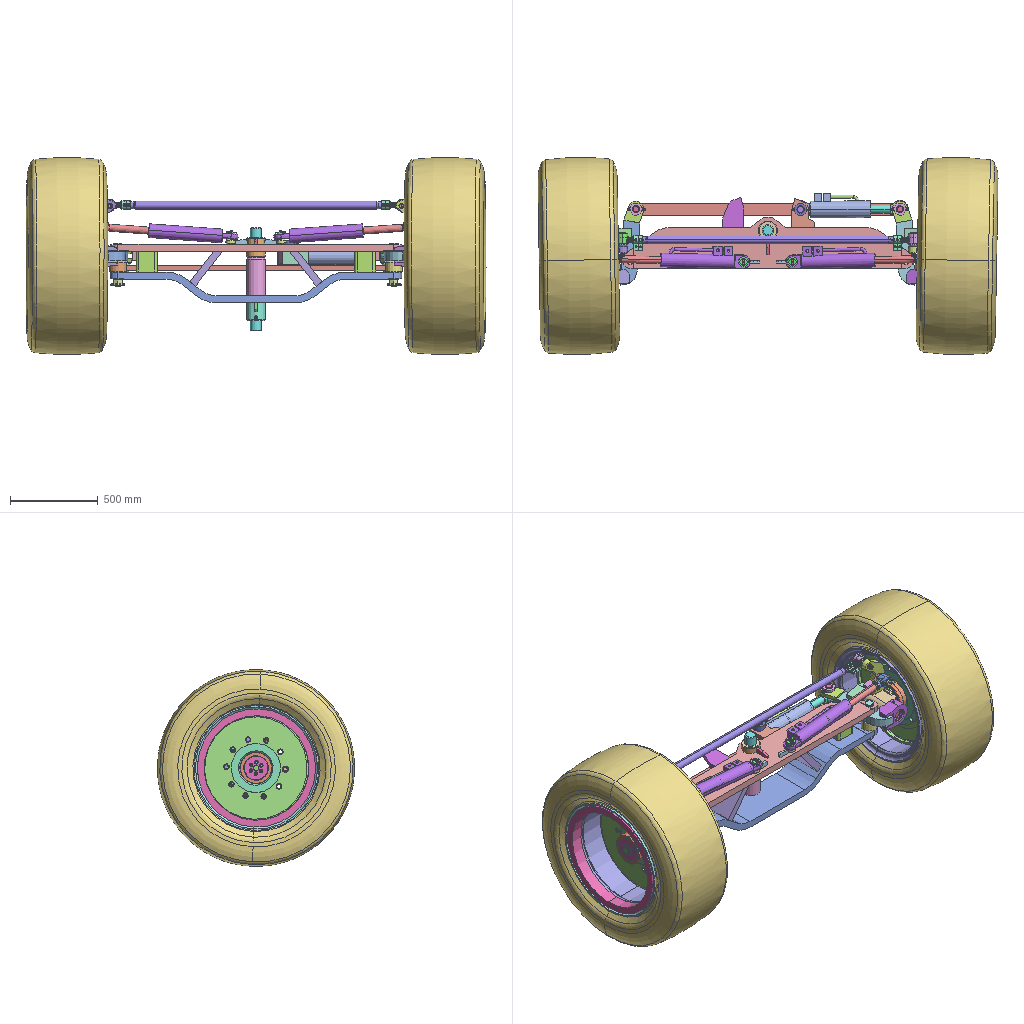Assembly | SolidWorks | 108 different items | 254 placed | box 2615 x 1120 x 1117 mm
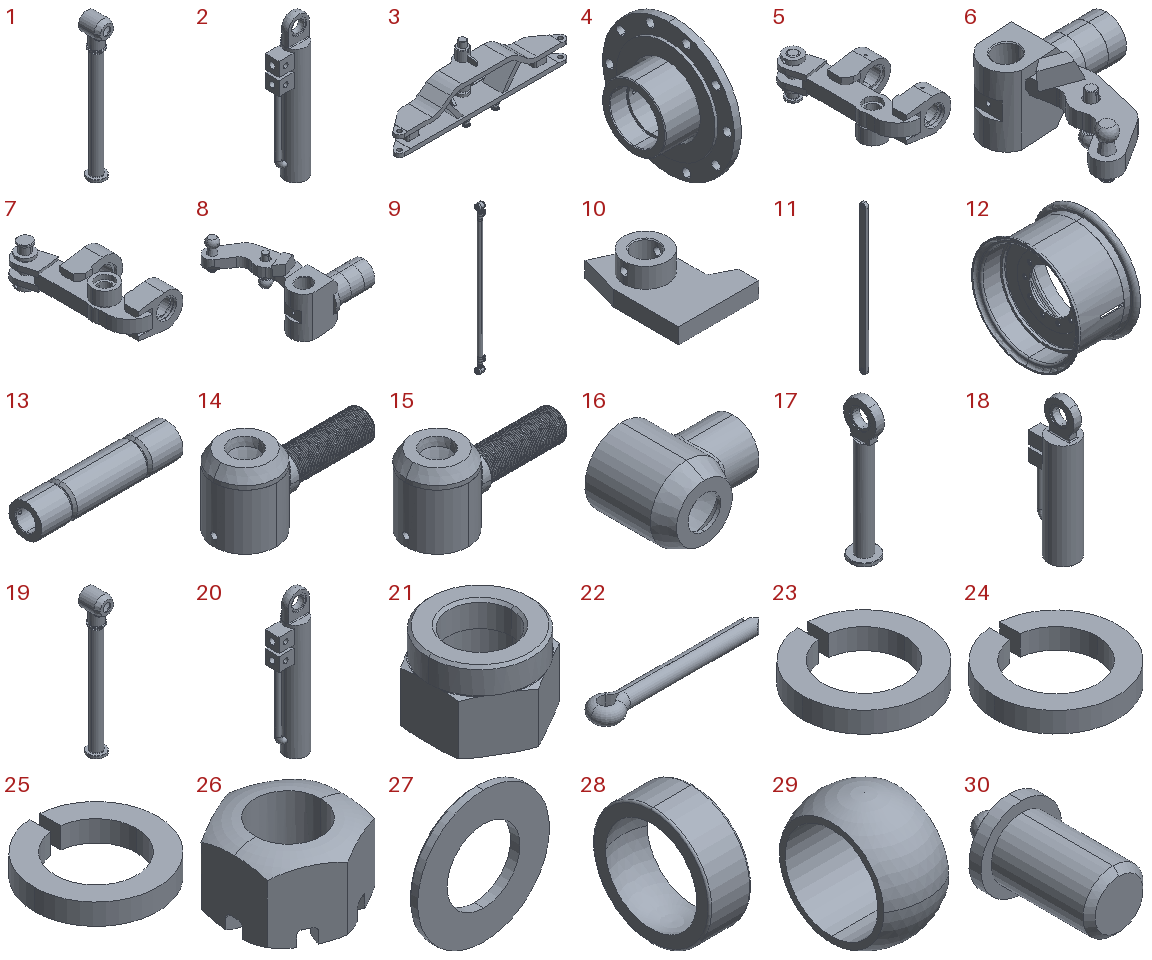Parts list (item | name | quantity | parent item | size | volume | features):
1 | (subassembly) | x1 | - | 65 x 84.5 x 521.5 mm | 755926 mm3 | features AEMSimFeature 1
2 | (subassembly) | x1 | - | 124 x 78 x 509 mm | 1093620 mm3 | features AEMSimFeature 1
3 | (subassembly) | x1 | - | 1658 x 403.509 x 586 mm | 38283555 mm3 | -
4 | (subassembly) | x2 | - | 164 x 375 x 375 mm | 3788319 mm3 | features AEMSimFeature 1
5 | (subassembly) | x1 | - | 241.001 x 479.989 x 157 mm | 4305652 mm3 | features Cut 2, RefAxis 2, RevCut 2, AEMSimFeature 1
6 | (subassembly) | x1 | - | 314 x 375 x 193.9 mm | 3181151 mm3 | features CompositeCurve 2, AEMSimFeature 1
7 | (subassembly) | x1 | - | 241.001 x 479.989 x 157 mm | 4310466 mm3 | features Cut 2, RefAxis 2, RevCut 2, AEMSimFeature 1
8 | (subassembly) | x1 | - | 314 x 375 x 193.9 mm | 3181178 mm3 | features CompositeCurve 2, AEMSimFeature 1
9 | (subassembly) | x1 | - | 103 x 64 x 1722 mm | 2094489 mm3 | features ReferencePattern 2, MirrorCompFeat 1
10 | (subassembly) | x1 | in 3 | 129 x 168.47 x 72 mm | 470442 mm3 | features AEMSimFeature 1
11 | (subassembly) | x1 | - | 30 x 77.5 x 1570 mm | 3189069 mm3 | features MirrorCompFeat 1, ReferencePattern 1
12 | (subassembly) | x2 | - | 410 x 711 x 711 mm | 14022631 mm3 | features AEMSimFeature 1
13 | (subassembly) | x1 | in 3 | 462 x 108 x 108 mm | 2151282 mm3 | features AEMSimFeature 1
14 | (subassembly) | x1 | in 9 | 152 x 64 x 82 mm | 214703 mm3 | -
15 | (subassembly) | x1 | in 9 | 152 x 64 x 82 mm | 214559 mm3 | -
16 | (subassembly) | x2 | in 1, 19 | 97.5 x 84.5 x 65 mm | 175742 mm3 | features AEMSimFeature 1
17 | (subassembly) | x1 | - | 80 x 100 x 410 mm | 667768 mm3 | features AEMSimFeature 1
18 | (subassembly) | x1 | - | 95 x 142.5 x 448 mm | 1129896 mm3 | features AEMSimFeature 1
19 | (subassembly) | x1 | - | 65 x 84.5 x 521.5 mm | 755926 mm3 | features AEMSimFeature 1
20 | (subassembly) | x1 | - | 124 x 78 x 509 mm | 1093620 mm3 | features AEMSimFeature 1
21 | - | x3 | - | 15.68 x 17.77 x 11.9 mm | 1480 mm3 | features Cut 3, Boss 1, Chamfer 1, Extrusion 1
22 | - | x2 | - | 83 x 15 x 8 mm | 4081 mm3 | features Cut 1, Sweep 1
23 | - | x12 | - | 18.367 x 18.334 x 3.1 mm | 444.091 mm3 | features Extrusion 1
24 | - | x2 | - | 30.149 x 30.097 x 5 mm | 1905 mm3 | features Extrusion 1
25 | - | x4 | - | 12.277 x 12.254 x 2.1 mm | 135.755 mm3 | features Extrusion 1
26 | - | x2 | - | 46 x 50.85 x 34.366 mm | 35234 mm3 | features CirPattern 1, Extrusion 1, Fillet 1, HoleWzd 1, ICE 1, RefAxis 1, RevCut 1
27 | - | x2 | - | 56 x 4 x 56 mm | 6746 mm3 | features Revolution 1
28 | - | x2 | in 17, 18 | 22 x 62 x 62 mm | 20588 mm3 | features Fillet 1, Revolution 1
29 | - | x2 | in 3, 5 | 28 x 53 x 53 mm | 20840 mm3 | features Revolution 1
30 | - | x8 | in 11 | 13.4 x 23.7 x 13.4 mm | 1610 mm3 | features Chamfer 1, Extrusion 1, ICE 1, Revolution 1
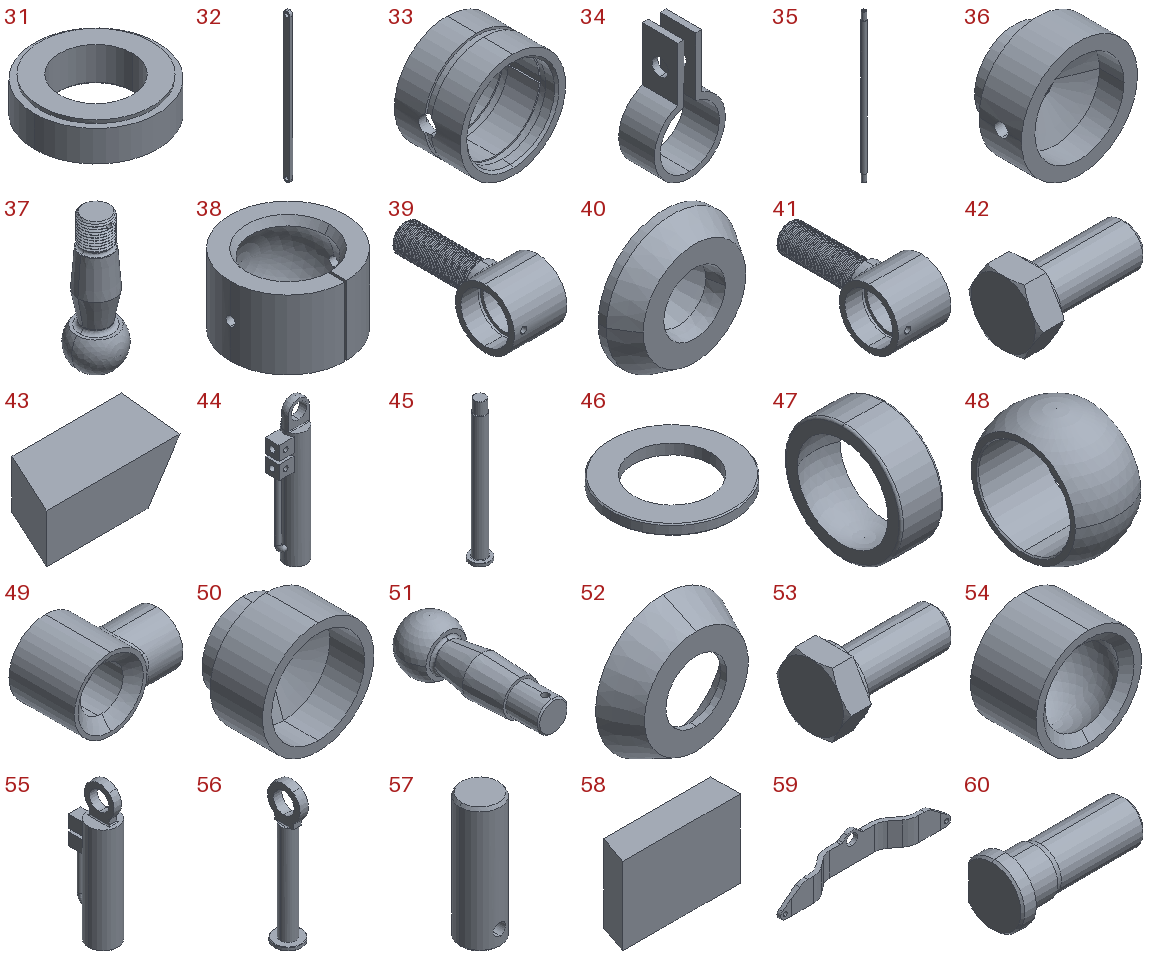31 | - | x4 | - | 68 x 68 x 19 mm | 43740 mm3 | features Chamfer 1, Extrusion 1, ICE 1, RevCut 1
32 | - | x1 | in 11 | 30 x 70 x 1570 mm | 3155166 mm3 | features Chamfer 1, Extrusion 1, HoleWzd 1
33 | - | x2 | in 11 | 48 x 30 x 48 mm | 15342 mm3 | features ICE 2, Chamfer 1, Extrusion 1, RevCut 1
34 | - | x4 | in 9 | 48 x 24 x 83 mm | 18610 mm3 | features Extrusion 1, ICE 1
35 | - | x1 | in 9 | 45 x 45 x 1535 mm | 1600076 mm3 | features ICE 5, HoleWzd 2, MirrorPattern 2, Chamfer 1, Extrusion 1
36 | - | x2 | in 14, 15 | 52 x 29 x 52 mm | 32471 mm3 | features HoleWzd 1, ICE 1, Revolution 1
37 | - | x2 | in 6, 8 | 40 x 40 x 108 mm | 69235 mm3 | features Chamfer 1, Helix 1, ICE 1, Revolution 1, SweepCut 1
38 | - | x2 | in 14, 15 | 50 x 49.995 x 30 mm | 27277 mm3 | features ICE 2, Revolution 1
39 | - | x1 | in 14 | 57 x 152 x 64 mm | 133317 mm3 | features ICE 2, Chamfer 1, Fillet 1, Helix 1, HoleWzd 1, Revolution 1, SweepCut 1
40 | - | x2 | in 14, 15 | 64 x 26 x 64 mm | 21380 mm3 | features Revolution 1
41 | - | x1 | in 15 | 57 x 152 x 64 mm | 133445 mm3 | features ICE 2, Chamfer 1, Fillet 1, Helix 1, HoleWzd 1, Revolution 1, SweepCut 1
42 | - | x2 | - | 57.5 x 34.641 x 30 mm | 23682 mm3 | features RevCut 4, Chamfer 1, Extrusion 1, Fillet 1, LPattern 1, Revolution 1
43 | - | x2 | in 8 | 86.452 x 40 x 30 mm | 78358 mm3 | features ICE 2, Extrusion 1
44 | - | x2 | in 2, 20 | 124 x 78 x 509 mm | 1078781 mm3 | features ICE 5, HoleWzd 2, RevCut 2, Chamfer 1, Extrusion 1, Fillet 1, MirrorPattern 1, Sweep 1
45 | - | x2 | in 1, 19 | 63 x 63 x 449 mm | 573468 mm3 | features Chamfer 2, ICE 2, Extrusion 1, Fillet 1
46 | - | x2 | in 1, 19 | 55 x 55 x 4.6 mm | 6709 mm3 | features Chamfer 1, Extrusion 1
47 | - | x2 | in 2, 20 | 20 x 55 x 55 mm | 14839 mm3 | features Fillet 1, Revolution 1
48 | - | x2 | in 3 | 25 x 47 x 47 mm | 15202 mm3 | features Chamfer 1, Revolution 1
49 | - | x2 | in 16 | 97.5 x 58.5 x 65 mm | 121615 mm3 | features RevCut 2, Fillet 1, ICE 1, RefAxis 1, Revolution 1
50 | - | x2 | in 16 | 48 x 32.5 x 48 mm | 28090 mm3 | features Revolution 1
51 | - | x2 | in 6, 8 | 40 x 109 x 40 mm | 70889 mm3 | features Chamfer 1, Fillet 1, ICE 1, Revolution 1
52 | - | x2 | in 16 | 65 x 16 x 65 mm | 11714 mm3 | features Revolution 1
53 | - | x4 | - | 25.3 x 15.011 x 13 mm | 1760 mm3 | features RevCut 4, Chamfer 1, Extrusion 1, Fillet 1, LPattern 1, Revolution 1
54 | - | x2 | in 16 | 45 x 28 x 45 mm | 14324 mm3 | features Revolution 1
55 | - | x1 | in 18 | - | - | features ICE 4, Chamfer 2, RevCut 2, Extrusion 1, Fillet 1, HoleWzd 1, SweepRefSurface 1
56 | - | x1 | in 17 | 80 x 100 x 410 mm | 647180 mm3 | features ICE 3, Chamfer 1, Extrusion 1, Fillet 1, RevCut 1
57 | - | x1 | in 3 | 40 x 40 x 124 mm | 150791 mm3 | features Chamfer 2, Extrusion 1, ICE 1
58 | - | x2 | in 3 | 80.4 x 20 x 53 mm | 81461 mm3 | features Extrusion 1
59 | - | x1 | in 3 | 1658 x 175.5 x 290 mm | 14232483 mm3 | features Fillet 4, ICE 4, Extrusion 1
60 | - | x20 | - | 69 x 28 x 32 mm | 29821 mm3 | features Chamfer 2, Fillet 1, ICE 1, Revolution 1
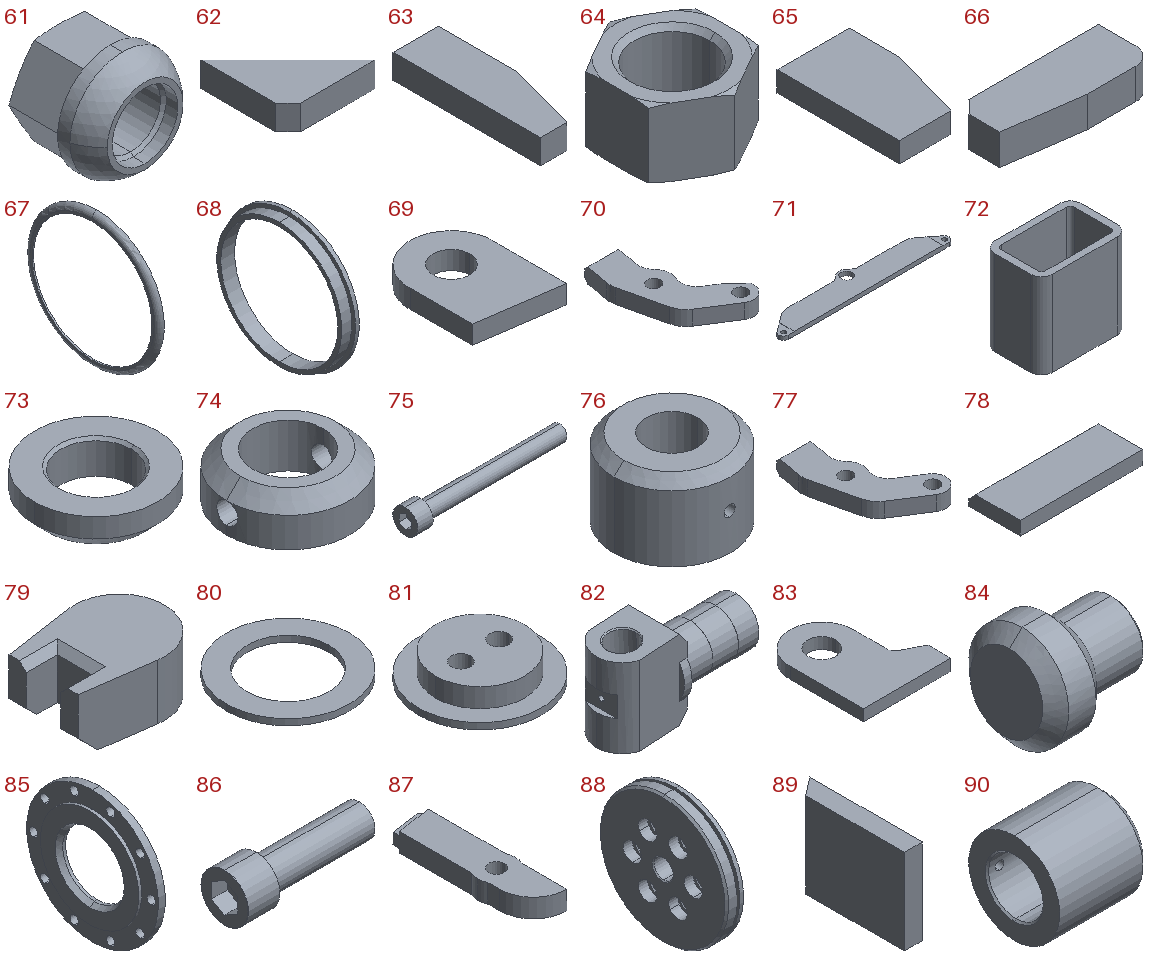61 | - | x20 | - | 36 x 30 x 36 mm | 14362 mm3 | features HoleWzd 1, ICE 1, RevCut 1, Revolution 1
62 | - | x1 | in 3 | 70 x 70 x 20 mm | 48000 mm3 | features Chamfer 1, Extrusion 1
63 | - | x1 | in 3 | 26 x 85 x 14 mm | 27860 mm3 | features Extrusion 1
64 | - | x3 | - | 17.386 x 20.03 x 10.8 mm | 1566 mm3 | features Cut 2, Chamfer 1, Extrusion 1
65 | - | x1 | in 3 | 50 x 85 x 14 mm | 54425 mm3 | features Extrusion 1
66 | - | x2 | in 3 | 65 x 25 x 14 mm | 21081 mm3 | features Chamfer 1, Extrusion 1, Fillet 1
67 | - | x2 | in 12 | 27 x 711 x 711 mm | 802010 mm3 | features Revolution 1
68 | - | x2 | in 12 | 70 x 672.4 x 672.4 mm | 3434576 mm3 | features Revolution 1
69 | - | x4 | in 5, 7 | 90 x 126 x 20 mm | 172239 mm3 | features Extrusion 1, ICE 1
70 | - | x1 | in 6 | 166.468 x 265 x 34 mm | 645452 mm3 | features Fillet 2, ICE 2, Chamfer 1, Extrusion 1
71 | - | x1 | in 3 | 1658 x 290 x 40 mm | 13542870 mm3 | features Fillet 2, ICE 2, Extrusion 1
72 | - | x2 | in 3 | 120 x 80 x 118 mm | 367424 mm3 | features Fillet 2, Extrusion 1
73 | - | x2 | in 5, 7 | 70 x 70 x 19 mm | 42599 mm3 | features Chamfer 2, Extrusion 1
74 | - | x2 | in 5, 7 | 70 x 70 x 25 mm | 54879 mm3 | features Chamfer 1, Extrusion 1, ICE 1
75 | - | x3 | - | 100 x 16 x 16 mm | 8793 mm3 | features BlendCut 1, Cut 1, Fillet 1, LPattern 1, RevCut 1, Revolution 1
76 | - | x2 | in 5, 7 | 95 x 95 x 62 mm | 343089 mm3 | features Chamfer 1, Extrusion 1, HoleWzd 1, ICE 1
77 | - | x1 | in 8 | 166.468 x 265 x 34 mm | 645456 mm3 | features Fillet 2, ICE 2, Chamfer 1, Extrusion 1
78 | - | x1 | in 3 | 180 x 75 x 20 mm | 261000 mm3 | features Chamfer 1, Extrusion 1
79 | - | x4 | in 5, 7 | 175 x 130 x 80 mm | 1338839 mm3 | features Chamfer 3, Extrusion 1
80 | - | x2 | in 3 | 100 x 100 x 5 mm | 22164 mm3 | features Extrusion 1
81 | - | x2 | in 3 | 58 x 58 x 12 mm | 18868 mm3 | features ICE 2, Extrusion 1
82 | - | x2 | in 6, 8 | 273 x 120 x 160.9 mm | 2317229 mm3 | features ICE 5, RefAxis 4, HoleWzd 3, RevCut 2, Chamfer 1, CirPattern 1, Extrusion 1, Fillet 1
83 | - | x1 | in 3 | 124 x 148.97 x 16 mm | 202996 mm3 | features Extrusion 1
84 | - | x2 | in 3 | 59.303 x 54 x 54 mm | 84349 mm3 | features Chamfer 2, RefAxis 2, HoleWzd 1, ICE 1, RefPoint 1, Revolution 1
85 | - | x2 | in 4 | 30 x 375 x 375 mm | 1925404 mm3 | features Chamfer 1, CirPattern 1, ICE 1, Revolution 1
86 | - | x12 | - | 52 x 18 x 18 mm | 7046 mm3 | features BlendCut 1, Cut 1, Fillet 1, LPattern 1, RevCut 1, Revolution 1
87 | - | x2 | in 5, 7 | 100 x 385 x 50 mm | 1537454 mm3 | features Extrusion 1, ICE 1
88 | - | x2 | - | 22 x 139 x 139 mm | 253971 mm3 | features Chamfer 3, CirPattern 1, RevCut 1, Revolution 1
89 | - | x2 | in 3 | 40 x 250.41 x 190 mm | 1785430 mm3 | features Extrusion 1
90 | - | x1 | in 13 | 107 x 108 x 108 mm | 551266 mm3 | features Chamfer 2, HoleWzd 1, Revolution 1
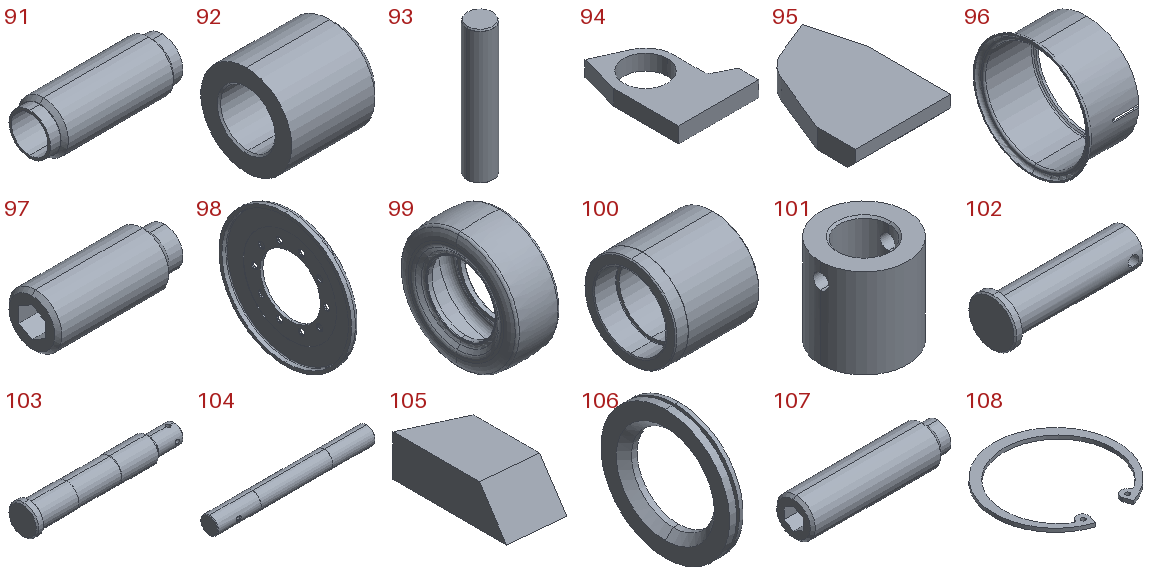91 | - | x1 | in 13 | 288 x 108 x 108 mm | 1046883 mm3 | features Chamfer 1, Revolution 1
92 | - | x1 | in 13 | 107 x 108 x 108 mm | 553133 mm3 | features Chamfer 2, Revolution 1
93 | - | x2 | - | 55 x 55 x 277 mm | 656436 mm3 | features Chamfer 2, HoleWzd 2, Extrusion 1, Fillet 1
94 | - | x1 | in 10 | 129 x 168.47 x 25 mm | 287390 mm3 | features Extrusion 1
95 | - | x1 | in 3 | 123 x 173.509 x 25 mm | 414715 mm3 | features Chamfer 1, Extrusion 1, Fillet 1
96 | - | x2 | in 12 | 340 x 711 x 711 mm | 6226699 mm3 | features Fillet 2, ICE 1, Revolution 1
97 | - | x2 | - | 30 x 12 x 12 mm | 2983 mm3 | features RevCut 2, Cut 1, LPattern 1, Revolution 1
98 | - | x2 | in 12 | 36 x 619 x 619 mm | 3559347 mm3 | features Fillet 2, Chamfer 1, CirPattern 1, ICE 1, RevCut 1, Revolution 1
99 | - | x2 | - | 450 x 1120 x 1120 mm | 112595756 mm3 | features RevCut 1, Revolution 1
100 | - | x2 | in 4 | 164 x 181 x 181 mm | 1862915 mm3 | features Chamfer 2, Fillet 1, HoleWzd 1, Revolution 1
101 | - | x1 | in 10 | 70 x 70 x 72 mm | 183051 mm3 | features Chamfer 1, Extrusion 1, ICE 1
102 | - | x2 | in 5, 7 | 154 x 54 x 54 mm | 196099 mm3 | features Chamfer 2, ICE 1, Revolution 1
103 | - | x2 | - | 246 x 46 x 48 mm | 282253 mm3 | features Chamfer 4, ICE 3, Revolution 1
104 | - | x1 | in 3 | 586 x 65 x 65 mm | 1913862 mm3 | features Chamfer 2, Fillet 1, HoleWzd 1, Revolution 1
105 | - | x2 | in 6 | 40 x 86.452 x 30 mm | 78358 mm3 | features ICE 2, Extrusion 1
106 | - | x2 | - | 14.5 x 139 x 139 mm | 109488 mm3 | features Revolution 1
107 | - | x1 | - | 45 x 12 x 12 mm | 4680 mm3 | features RevCut 2, Cut 1, LPattern 1, Revolution 1
108 | - | x4 | - | 85.5 x 83.408 x 2.5 mm | 3180 mm3 | features Extrusion 1
Mates (type | each side: item.copy, entity, surface, feature):
In the top assembly
Concentric | 71.1 face cylinder Boss-Extrude1 | 87.1 face cylinder Cut-Revolve1
DistanceDim | 87.1 face plane | 71.1 face plane Cut-Extrude1
Concentric | 71.1 face cylinder Boss-Extrude1 | 87.2 face cylinder Cut-Revolve1
DistanceDim | 87.2 face plane | 71.1 face plane Cut-Extrude1
Coincident | 55.1 plane | 56.1 plane
Concentric | 55.1 face cylinder Cut-Revolve1 | 56.1 face cylinder Boss-Extrude1
Concentric | 29.1 face sphere Revolve1 | 28.1 face sphere Revolve1
Concentric | 29.2 face sphere Revolve1 | 28.2 face sphere Revolve1
Concentric | 85.1 face cylinder Revolve1 | 98.1 face cylinder Revolve1
Coincident | 85.1 face plane Revolve1 | 98.1 face plane Revolve1
Concentric | 85.1 face cylinder Cut-Extrude1 | 98.1 face cylinder Cut-Extrude1
Concentric | 100.1 face cylinder Revolve1 | 98.2 face cylinder Revolve1
Concentric | 85.2 face cylinder Cut-Extrude1 | 98.2 face cylinder Cut-Extrude1
Coincident | 85.2 face plane Revolve1 | 98.2 face plane Revolve1
Concentric | 85.2 face cylinder Pattern(Circular)1 | 98.2 face cylinder Pattern(Circular)1
Concentric | 96.1 face cylinder Revolve1 | 99.1 face cylinder Revolve1
Coincident | 12.1 plane | 99.1 plane
Coincident | 67.1 plane | 99.1 plane
Concentric | 96.2 face cylinder Revolve1 | 99.2 face cylinder Revolve1
Coincident | 12.2 plane | 99.2 plane
Coincident | 67.2 plane | 99.2 plane
Concentric | 48.1 face sphere Revolve1 | 47.1 face sphere Revolve1
Concentric | 44.1 face cylinder Cut-Revolve1 | 45.1 face cylinder Boss-Extrude1
Concentric | 48.2 face sphere Revolve1 | 47.2 face sphere Revolve1
Coincident | 44.1 plane | 49.1 plane
Concentric | 102.1 face cylinder Revolve1 | 33.1 face cylinder Boss-Extrude1
Concentric | 102.2 face cylinder Revolve1 | 33.2 face cylinder Boss-Extrude1
Coincident | 73.1 face plane Boss-Extrude1 | 32.1 face plane Boss-Extrude1
Concentric | 79.1 face cylinder Cut-Revolve3 | 82.1 face cylinder Cut-Revolve2
Concentric | 79.2 face cylinder Cut-Revolve2 | 82.2 face cylinder Cut-Revolve2
DistanceDim | 82.1 face plane Cut-Extrude1 | 79.1 face plane Cut-Extrude3
DistanceDim | 82.2 face plane Cut-Extrude1 | 79.2 face plane Cut-Extrude3
Concentric | 82.1 face cylinder Boss-Extrude3 | 100.2 face cylinder Revolve1
Coincident | 82.1 plane | 100.2 plane
DistanceDim | 85.1 face plane Revolve1 | 82.1 face plane Boss-Extrude1
Concentric | 82.2 face cylinder Boss-Extrude3 | 100.1 face cylinder Revolve1
Coincident | 82.2 plane | 100.1 plane
DistanceDim | 85.2 face plane Revolve1 | 82.2 face plane Boss-Extrude1
Concentric | 44.2 face cylinder Cut-Revolve1 | 45.2 face cylinder Boss-Extrude1
Coincident | 44.2 plane | 45.2 plane
Concentric | 51.1 face sphere Revolve1 | 54.1 face sphere Revolve1
Concentric | 51.2 face sphere Revolve1 | 54.2 face sphere Revolve1
Concentric | 82.1 face cylinder Cut-Revolve2 | 93.1 face cylinder Boss-Extrude1
Concentric | 82.1 face cylinder M12x1.5 ThreadHole2 | 93.1 face cylinder Size mm Dowel PinHole2
Concentric | 82.2 face cylinder Cut-Revolve2 | 93.2 face cylinder Boss-Extrude1
Concentric | 82.2 face cylinder M12x1.5 ThreadHole2 | 93.2 face cylinder Size mm Dowel PinHole2
Concentric | 82.2 face cylinder M12x1.5 ThreadHole2 | 97.1 face cylinder Base-Revolve
Coincident | 82.2 plane | 97.1 plane
DistanceDim | 97.1 face plane Base-Revolve | 82.2 plane
Concentric | 82.1 face cylinder M12x1.5 ThreadHole2 | 97.2 face cylinder Base-Revolve
Coincident | 82.1 plane | 97.2 plane
DistanceDim | 97.2 face plane Base-Revolve | 82.1 plane
Concentric | 82.1 face cylinder Boss-Extrude3 | 106.1 face cylinder Revolve1
Coincident | 82.1 plane | 106.1 plane
Coincident | 82.1 face plane Boss-Extrude1 | 106.1 face plane Revolve1
Concentric | 82.2 face cylinder Boss-Extrude3 | 106.2 face cylinder Revolve1
Coincident | 82.2 plane | 106.2 plane
Coincident | 82.2 face plane Boss-Extrude1 | 106.2 face plane Revolve1
Concentric | 100.2 face cylinder Revolve1 | 88.1 face cylinder Revolve1
Concentric | 82.1 face cylinder Pattern(Circular)1 | 88.1 face cylinder Cut-Revolve1
Coincident | 82.1 face plane Boss-Extrude3 | 88.1 face plane Revolve1
Concentric | 100.1 face cylinder Revolve1 | 88.2 face cylinder Revolve1
Concentric | 82.2 face cylinder Pattern(Circular)1 | 88.2 face cylinder Pattern(Circular)1
Coincident | 82.2 face plane Boss-Extrude3 | 88.2 face plane Revolve1
Coincident | 71.1 axis | 103.1 axis
Coincident | 71.1 face plane Cut-Extrude1 | 103.1 face plane Revolve1
Parallel | 71.1 face plane Cut-Extrude1 | 103.1 face plane Cut-Extrude1
Concentric | 71.1 face cylinder Boss-Extrude1 | 103.2 face cylinder Revolve1
Coincident | 71.1 face plane Cut-Extrude1 | 103.2 face plane Revolve1
Parallel | 71.1 face plane Cut-Extrude1 | 103.2 face plane Cut-Extrude1
Concentric | 85.1 face cylinder Pattern(Circular)1 | 60.1 face cylinder Revolve1
Coincident | 82.1 plane | 60.1 plane
Coincident | 85.1 face plane Revolve1 | 60.1 face plane Revolve1
Concentric | 60.1 face cylinder Revolve1 | 61.1 face cylinder M22x1.5 ThreadHole1
Coincident | 82.1 plane | 61.1 plane
Concentric | 98.1 face sphere Pattern(Circular)1 | 61.1 face sphere Revolve1
Coincident | 82.2 plane | 60.2 plane
Concentric | 85.2 face cylinder Pattern(Circular)1 | 60.2 face cylinder Revolve1
Coincident | 85.2 face plane Revolve1 | 60.2 face plane Revolve1
Coincident | 82.2 plane | 61.2 plane
Concentric | 60.2 face cylinder Revolve1 | 61.2 face cylinder M22x1.5 ThreadHole1
Concentric | 98.2 face sphere Pattern(Circular)1 | 61.2 face sphere Revolve1
Coincident | 81.1 plane | 25.1 plane
Concentric | 81.1 face cylinder Cut-Extrude1 | 25.1 face cylinder Extrude1
Coincident | 81.1 face plane Boss-Extrude1 | 25.1 face plane Extrude1
Coincident | 81.1 face plane Boss-Extrude1 | 25.2 face plane Extrude1
Coincident | 81.1 plane | 25.2 plane
Concentric | 81.1 face cylinder Cut-Extrude1 | 25.2 face cylinder Extrude1
Coincident | 81.2 face plane Boss-Extrude1 | 25.3 face plane Extrude1
Coincident | 81.2 plane | 25.3 plane
Concentric | 81.2 face cylinder Cut-Extrude1 | 25.3 face cylinder Extrude1
Coincident | 81.2 face plane Boss-Extrude1 | 25.4 face plane Extrude1
Coincident | 81.2 plane | 25.4 plane
Concentric | 81.2 face cylinder Cut-Extrude1 | 25.4 face cylinder Extrude1
Coincident | 25.1 face plane Extrude1 | 53.1 face plane Base-Extrude
Coincident | 81.1 plane | 53.1 plane
Concentric | 25.1 face cylinder Extrude1 | 53.1 face cylinder Boss-Revolve1
Coincident | 25.2 face plane Extrude1 | 53.2 face plane Base-Extrude
Coincident | 53.1 plane | 53.2 plane
Concentric | 25.2 face cylinder Extrude1 | 53.2 face cylinder Boss-Revolve1
Coincident | 25.3 face plane Extrude1 | 53.3 face plane Base-Extrude
Coincident | 81.2 plane | 53.3 plane
Concentric | 25.3 face cylinder Extrude1 | 53.3 face cylinder Boss-Revolve1
Coincident | 25.4 face plane Extrude1 | 53.4 face plane Base-Extrude
Coincident | 81.2 plane | 53.4 plane
Concentric | 25.4 face cylinder Extrude1 | 53.4 face cylinder Boss-Revolve1
Concentric | 79.1 face cylinder Cut-Extrude4 | 30.1 face cylinder Boss-Extrude2
Coincident | 79.1 plane | 30.1 plane
DistanceDim | 30.1 face plane Boss-Extrude1 | 87.1 plane
Concentric | 79.3 face cylinder Cut-Extrude4 | 30.2 face cylinder Boss-Extrude2
Coincident | 79.3 plane | 30.2 plane
DistanceDim | 30.2 face plane Boss-Extrude1 | 79.3 plane
Concentric | 79.2 face cylinder Cut-Extrude4 | 30.3 face cylinder Boss-Extrude2
Coincident | 79.2 plane | 30.3 plane
DistanceDim | 30.3 face plane Boss-Extrude1 | 79.2 plane
Concentric | 79.4 face cylinder Cut-Extrude4 | 30.4 face cylinder Boss-Extrude2
Coincident | 79.4 plane | 30.4 plane
DistanceDim | 30.4 face plane Boss-Extrude1 | 79.2 plane
Coincident | 100.2 plane | 30.5 plane
Concentric | 100.2 face cylinder M10x1.0 ThreadHole2 | 30.5 face cylinder Boss-Extrude2
DistanceDim | 30.5 face plane Boss-Extrude1 | 100.2 plane
Coincident | 100.1 plane | 30.6 plane
DistanceDim | 30.6 face plane Boss-Extrude1 | 100.1 plane
Concentric | 100.1 face cylinder M10x1.0 ThreadHole2 | 30.6 face cylinder Boss-Extrude2
Coincident | 59.1 face plane Cut-Extrude3 | 27.1 face plane Base-Revolve
Coincident | 103.2 plane | 27.1 plane
Concentric | 103.2 face cylinder Revolve1 | 27.1 face cylinder Base-Revolve
Coincident | 103.2 plane | 26.1 plane
Concentric | 103.2 face cylinder Revolve1 | 26.1 face cylinder M30x2.0 ThreadHole1
Coincident | 27.1 face plane Base-Revolve | 26.1 edge
Coincident | 103.1 plane | 27.2 plane
Concentric | 103.1 face cylinder Revolve1 | 27.2 face cylinder Base-Revolve
Coincident | 59.1 face plane Cut-Extrude3 | 27.2 face plane Base-Revolve
Coincident | 103.1 plane | 26.2 plane
Concentric | 103.1 face cylinder Revolve1 | 26.2 face cylinder M30x2.0 ThreadHole1
Coincident | 27.2 face plane Base-Revolve | 26.2 edge
Coincident | 103.2 plane | 22.1 plane
DistanceDim | 22.1 plane | 103.2 plane
Concentric | 103.2 face cylinder Cut-Extrude2 | 22.1 face cylinder Body
DistanceDim | 22.2 plane | 103.1 plane
Coincident | 103.1 plane | 22.2 plane
Concentric | 103.1 face cylinder Cut-Extrude2 | 22.2 face cylinder Body
Parallel | 107.1 plane | 91.1 plane
Concentric | 90.1 face cylinder M12x1.25 ThreadHole1 | 107.1 face cylinder Base-Revolve
DistanceDim | 107.1 face plane Base-Revolve | 104.1 plane
Concentric | 107.1 face cylinder Base-Revolve | 64.1 face cylinder Base-Extrude
Coincident | 80.1 plane | 64.1 plane
DistanceDim | 91.1 plane | 64.1 face plane Base-Extrude
Coincident | 97.2 plane | 64.2 plane
Concentric | 97.2 face cylinder Base-Revolve | 64.2 face cylinder Base-Extrude
DistanceDim | 64.2 face plane Base-Extrude | 97.2 face plane Base-Revolve
Coincident | 97.1 plane | 64.3 plane
Concentric | 97.1 face cylinder Base-Revolve | 64.3 face cylinder Base-Extrude
DistanceDim | 64.3 face plane Base-Extrude | 97.1 face plane Base-Revolve
Coincident | 82.1 plane | 24.1 plane
Concentric | 88.1 face cylinder Revolve1 | 24.1 face cylinder Extrude1
Coincident | 88.1 face plane Revolve1 | 24.1 face plane Extrude1
Coincident | 82.2 plane | 24.2 plane
Coincident | 88.2 face plane Revolve1 | 24.2 face plane Extrude1
Concentric | 88.2 face cylinder Revolve1 | 24.2 face cylinder Extrude1
Concentric | 24.1 face cylinder Extrude1 | 42.1 face cylinder Boss-Revolve1
Coincident | 24.1 plane | 42.1 plane
Coincident | 24.1 face plane Extrude1 | 42.1 face plane Base-Extrude
Coincident | 24.2 plane | 42.2 plane
Coincident | 24.2 face plane Extrude1 | 42.2 face plane Base-Extrude
Concentric | 24.2 face cylinder Extrude1 | 42.2 face cylinder Boss-Revolve1
Coincident | 88.1 face plane Cut-Revolve1 | 23.1 edge
Coincident | 88.1 plane | 23.1 plane
Concentric | 88.1 face cylinder Cut-Revolve1 | 23.1 face cylinder Extrude1
Coincident | 88.1 plane | 86.1 plane
Coincident | 23.1 face plane Extrude1 | 86.1 face plane Base-Revolve
Concentric | 23.1 face cylinder Extrude1 | 86.1 face cylinder Base-Revolve
Coincident | 88.2 face plane Cut-Revolve1 | 23.2 face plane Extrude1
Concentric | 88.2 face cylinder Cut-Revolve1 | 23.2 face cylinder Extrude1
Coincident | 88.2 plane | 23.2 plane
Concentric | 88.2 face cylinder Cut-Revolve1 | 86.2 face cylinder Base-Revolve
Coincident | 23.2 plane | 86.2 plane
Coincident | 23.2 face plane Extrude1 | 86.2 face plane Base-Revolve
Coincident | 79.3 plane | 108.1 plane
Coincident | 79.1 face plane Cut-Revolve3 | 108.1 face plane Base-Extrude
Concentric | 79.1 face cylinder Cut-Revolve3 | 108.1 face cylinder Base-Extrude
Coincident | 79.4 plane | 108.2 plane
Coincident | 79.2 face plane Cut-Revolve2 | 108.2 face plane Base-Extrude
Concentric | 79.2 face cylinder Cut-Revolve2 | 108.2 face cylinder Base-Extrude
Coincident | 79.1 plane | 108.3 plane
Coincident | 79.3 face plane Cut-Revolve3 | 108.3 face plane Base-Extrude
Concentric | 79.3 face cylinder Cut-Revolve3 | 108.3 face cylinder Base-Extrude
Coincident | 79.2 plane | 108.4 plane
Coincident | 79.4 face plane Cut-Revolve2 | 108.4 face plane Base-Extrude
Concentric | 79.4 face cylinder Cut-Revolve2 | 108.4 face cylinder Base-Extrude
Concentric | 74.1 face cylinder Cut-Extrude1 | 75.1 face cylinder Base-Revolve
DistanceDim | 75.1 face plane Base-Revolve | 102.1 plane
Coincident | 29.1 plane | 75.2 plane
Concentric | 101.1 face cylinder Cut-Extrude1 | 75.2 face cylinder Base-Revolve
DistanceDim | 75.2 face plane Base-Revolve | 57.1 plane
Concentric | 74.2 face cylinder Cut-Extrude1 | 75.3 face cylinder Base-Revolve
Coincident | 74.2 plane | 75.3 plane
DistanceDim | 75.3 face plane Base-Revolve | 74.2 plane
Coincident | 102.1 plane | 75.1 plane
Coincident | 75.1 plane | 21.1 plane
Concentric | 75.1 face cylinder Base-Revolve | 21.1 face cylinder Cut-Extrude3
DistanceDim | 21.1 face plane Base-Extrude | 74.1 plane
Coincident | 75.2 plane | 21.2 plane
Concentric | 75.2 face cylinder Base-Revolve | 21.2 face cylinder Base-Extrude
DistanceDim | 21.2 face plane Base-Extrude | 57.1 plane
Coincident | 75.3 plane | 21.3 plane
Concentric | 75.3 face cylinder Base-Revolve | 21.3 face cylinder Cut-Extrude3
DistanceDim | 21.3 face plane Base-Extrude | 102.2 plane
Concentric | 37.1 face sphere Revolve2 | 38.1 face sphere Revolve1
Concentric | 37.2 face sphere Revolve2 | 38.2 face sphere Revolve1
Coincident | 70.1 face plane Boss-Extrude1 | 105.1 face plane Boss-Extrude1
DistanceDim | 105.1 vertex | 70.1 face plane Boss-Extrude1 | 2 times
DistanceDim | 105.1 vertex | 82.2 face plane Boss-Extrude1
Coincident | 77.1 face plane Boss-Extrude1 | 43.1 face plane Boss-Extrude1
DistanceDim | 43.1 vertex | 77.1 face plane Boss-Extrude1 | 2 times
DistanceDim | 43.1 vertex | 82.1 face plane Boss-Extrude1
Coincident | 103.1 plane | 31.1 plane
Coincident | 76.1 face plane Cut-Revolve1 | 31.1 face plane Boss-Extrude1
Concentric | 103.1 face cylinder Revolve1 | 31.1 face cylinder Cut-Extrude1
Coincident | 87.1 face plane Cut-Revolve1 | 31.2 face plane Boss-Extrude1
Coincident | 103.1 plane | 31.2 plane
Concentric | 103.1 face cylinder Revolve1 | 31.2 face cylinder Cut-Extrude1
Coincident | 76.2 face plane Cut-Revolve1 | 31.3 face plane Boss-Extrude1
Coincident | 103.2 plane | 31.3 plane
Concentric | 103.2 face cylinder Revolve1 | 31.3 face cylinder Cut-Extrude1
Coincident | 103.2 plane | 31.4 plane
Concentric | 103.2 face cylinder Revolve1 | 31.4 face cylinder Cut-Extrude1
Coincident | 87.2 face plane Cut-Revolve1 | 31.4 face plane Boss-Extrude1
PlanarAngleDim | 87.2 face plane | 71.1 face plane Boss-Extrude1
Parallel | 71.1 face plane Boss-Extrude1 | 9.1 plane
In subassembly 4
Concentric | 85.3 face cylinder Revolve1 | 100.3 face cylinder Revolve1
DistanceDim | 100.3 face plane Revolve1 | 85.3 face plane Revolve1
Coincident | 85.3 plane | 100.3 plane
In subassembly 17
Concentric | 56.2 face cylinder Cut-Extrude1 | 28.3 face cylinder Revolve1
Coincident | 56.2 plane | 28.3 plane | 2 times
In subassembly 9
Coincident | 35.1 axis | 39.1 axis
Coincident | 35.1 axis | 41.1 axis
Coincident | 35.1 axis | 34.1 plane
Parallel | 35.1 plane | 34.1 plane
Coincident | 35.1 axis | 34.1 axis
Coincident | 35.1 axis | 34.2 plane
Parallel | 35.1 plane | 34.2 plane
Coincident | 35.1 axis | 34.2 axis
Coincident | 35.1 plane | 9.2 plane | 3 times
DistanceDim | 35.1 plane | 39.1 plane
Coincident | 38.3 plane | 9.2 plane
Coincident | 36.1 plane | 9.2 plane
DistanceDim | 38.4 plane | 35.1 plane
In subassembly 14
Coincident | 39.2 face plane Revolve1 | 40.1 face plane Revolve1 | 2 times
Concentric | 39.2 face cylinder Revolve1 | 38.5 face cylinder Revolve1
Coincident | 39.2 plane | 38.5 plane
Coincident | 39.2 face plane Revolve1 | 38.5 face plane Revolve1
Coincident | 39.2 plane | 36.2 plane
Coincident | 38.5 face plane Revolve1 | 36.2 face plane Revolve1
Concentric | 39.2 face cylinder Revolve1 | 36.2 face cylinder Revolve1
Coincident | 39.2 plane | 40.1 plane
Concentric | 39.2 face cylinder Revolve1 | 40.1 face cylinder Revolve1
In subassembly 15
Coincident | 41.2 face plane Revolve1 | 40.1 face plane Revolve1 | 2 times
Coincident | 41.2 plane | 38.5 plane
Coincident | 41.2 face plane Revolve1 | 38.5 face plane Revolve1
Concentric | 41.2 face cylinder Revolve1 | 38.5 face cylinder Revolve1
Coincident | 38.5 face plane Revolve1 | 36.2 face plane Revolve1
Coincident | 41.2 plane | 36.2 plane
Concentric | 41.2 face cylinder Revolve1 | 36.2 face cylinder Revolve1
Coincident | 41.2 plane | 40.1 plane
Concentric | 41.2 face cylinder Revolve1 | 40.1 face cone Revolve1
In subassembly 5
Coincident | 87.3 face plane | 69.1 face plane Boss-Extrude1 | 2 times
Coincident | 87.3 face plane | 69.1 edge
Coincident | 87.3 face plane | 79.5 face plane
Coincident | 87.3 plane | 79.5 plane
DistanceDim | 79.5 face plane | 87.3 plane
Coincident | 87.3 plane | 79.6 plane
DistanceDim | 79.6 face plane | 87.3 plane
Coincident | 87.3 face plane | 79.6 face plane
DistanceDim | 74.3 plane | 87.3 plane
Coincident | 69.1 face plane Boss-Extrude1 | 73.2 face plane Boss-Extrude1
DistanceDim | 73.2 plane | 87.3 plane
DistanceDim | 74.3 plane | 87.3 face plane
DistanceDim | 73.2 plane | 87.3 face plane
Coincident | 87.3 face plane | 76.3 face plane
Concentric | 87.3 face cylinder Boss-Extrude1 | 76.3 face cylinder Boss-Extrude1
Parallel | 87.3 face plane | 76.3 plane
Concentric | 74.3 face cylinder Cut-Extrude1 | 102.3 face cylinder Cut-Extrude1
Parallel | 73.2 face cylinder Boss-Extrude1 | 102.3 face cylinder Revolve1
Coincident | 73.2 plane | 102.3 plane
Concentric | 102.3 face cylinder Revolve1 | 29.3 face cylinder Revolve1
DistanceDim | 29.3 face plane Revolve1 | 69.1 face plane Boss-Extrude1
Coincident | 87.3 face plane | 69.2 face plane Boss-Extrude1 | 2 times
Coincident | 87.3 face plane | 69.2 edge
Parallel | 76.3 plane | 102.3 plane
Coincident | 69.2 face plane Boss-Extrude1 | 74.3 face plane Boss-Extrude1
In subassembly 18
Concentric | 55.2 face cylinder Cut-Extrude2 | 28.3 face cylinder Revolve1
Coincident | 55.2 plane | 28.3 plane | 2 times
In subassembly 2
Concentric | 44.3 face cylinder Cut-Extrude3 | 47.3 face cylinder Revolve1
Coincident | 44.3 plane | 47.3 plane | 2 times
In subassembly 19
Concentric | 45.3 face cylinder Boss-Extrude3 | 49.2 face cylinder Cut-Revolve2
Coincident | 45.3 plane | 49.2 plane
DistanceDim | 45.3 face plane Boss-Extrude3 | 54.3 plane
Coincident | 49.2 plane | 46.1 plane
Coincident | 49.2 face plane Boss-Extrude1 | 46.1 face plane Boss-Extrude1
Concentric | 45.3 face cylinder Boss-Extrude3 | 46.1 face cylinder Boss-Extrude1
In subassembly 16
Coincident | 49.3 face plane Revolve1 | 52.1 face plane Revolve1
Coincident | 49.3 plane | 54.4 plane
Coincident | 49.3 face plane Cut-Revolve1 | 54.4 face plane Revolve1
Concentric | 49.3 face cylinder Cut-Revolve1 | 54.4 face cylinder Revolve1
Coincident | 49.3 plane | 52.1 plane
Concentric | 49.3 face cylinder Revolve1 | 52.1 face cylinder Revolve1
Coincident | 50.1 plane | 54.4 plane
Coincident | 49.3 face plane Cut-Revolve1 | 50.1 face plane Revolve1
Concentric | 49.3 face cylinder Cut-Revolve1 | 50.1 face cylinder Revolve1
In subassembly 3
Coincident | 71.2 face plane Boss-Extrude1 | 78.1 face plane Boss-Extrude1
DistanceDim | 78.1 face plane Boss-Extrude1 | 71.2 plane
Coincident | 71.2 face plane Boss-Extrude1 | 84.1 face plane Cut-Extrude1 | 2 times
DistanceDim | 89.1 edge | 71.2 plane
DistanceDim | 89.2 edge | 71.2 plane
Coincident | 71.2 plane | 59.2 plane
Concentric | 71.2 face cylinder Boss-Extrude1 | 59.2 face cylinder Cut-Extrude1
DistanceDim | 59.2 face plane Boss-Extrude1 | 71.2 face plane Boss-Extrude1
Coincident | 71.2 face plane Boss-Extrude1 | 72.1 face plane Boss-Extrude1
DistanceDim | 72.1 plane | 59.2 plane
DistanceDim | 72.2 plane | 71.2 plane
Coincident | 71.2 face plane Boss-Extrude1 | 72.2 face plane Boss-Extrude1
Coincident | 71.2 plane | 91.2 plane
Concentric | 59.2 face cylinder Cut-Extrude1 | 90.2 face cylinder Revolve1
DistanceDim | 71.2 face plane Boss-Extrude1 | 92.1 face plane Revolve1
DistanceDim | 65.1 face plane Boss-Extrude1 | 59.2 plane
Coincident | 59.2 face plane Boss-Extrude1 | 89.2 face plane Boss-Extrude1
DistanceDim | 89.2 face plane Boss-Extrude1 | 59.2 face plane Cut-Extrude1
Coincident | 59.2 face plane Boss-Extrude1 | 89.1 face plane Boss-Extrude1
DistanceDim | 89.1 face plane Boss-Extrude1 | 59.2 face plane Cut-Extrude1
Coincident | 59.2 face plane Boss-Extrude1 | 65.1 face plane Boss-Extrude1
Tangent | 90.2 face cylinder Revolve1 | 65.1 face plane Boss-Extrude1
DistanceDim | 84.1 plane | 91.2 plane
DistanceDim | 84.1 point | 71.2 plane
Coincident | 71.2 face plane Boss-Extrude1 | 84.2 face plane Cut-Extrude1
DistanceDim | 84.2 plane | 91.2 plane
DistanceDim | 84.2 point | 71.2 plane
DistanceDim | 59.2 face plane Cut-Extrude1 | 72.2 face plane Boss-Extrude1
DistanceDim | 59.2 face plane Cut-Extrude1 | 72.1 face plane Boss-Extrude1
Coincident | 89.2 face plane Boss-Extrude1 | 78.1 face plane Boss-Extrude1
Concentric | 101.2 face cylinder Boss-Extrude1 | 83.1 face cylinder Boss-Extrude1
DistanceDim | 71.2 face plane Boss-Extrude1 | 94.1 face plane Boss-Extrude1
DistanceDim | 83.1 face plane Boss-Extrude1 | 101.2 face plane Boss-Extrude1
DistanceDim | 101.2 plane | 71.2 plane
DistanceDim | 101.2 plane | 91.2 plane
Coincident | 101.2 plane | 83.1 plane
DistanceDim | 95.1 face plane Boss-Extrude1 | 71.2 face plane Boss-Extrude1
Coincident | 71.2 face plane Boss-Extrude1 | 62.1 face plane Boss-Extrude1
Coincident | 78.1 face plane Boss-Extrude1 | 62.1 face plane Boss-Extrude1
DistanceDim | 62.1 face plane Boss-Extrude1 | 101.2 plane
Concentric | 90.2 face cylinder Revolve1 | 104.2 face cylinder Revolve1
Concentric | 90.2 face cylinder M12x1.25 ThreadHole1 | 104.2 face cylinder Size mm Dowel PinHole2
Coincident | 71.2 plane | 80.2 plane
Coincident | 92.1 face plane Revolve1 | 80.2 face plane Boss-Extrude1
Concentric | 92.1 face cylinder Revolve1 | 80.2 face cylinder Boss-Extrude1
Coincident | 90.2 face plane Revolve1 | 80.3 face plane Boss-Extrude1
Coincident | 59.2 plane | 80.3 plane
Concentric | 90.2 face cylinder Revolve1 | 80.3 face cylinder Boss-Extrude1
Concentric | 101.2 face cylinder Boss-Extrude1 | 57.2 face cylinder Boss-Extrude1
Concentric | 101.2 face cylinder Cut-Extrude1 | 57.2 face cylinder Cut-Extrude2
Concentric | 57.2 face cylinder Boss-Extrude1 | 29.3 face cylinder Revolve1
Coincident | 101.2 plane | 29.3 plane
DistanceDim | 29.3 face plane Revolve1 | 101.2 face plane Boss-Extrude1
Concentric | 84.1 face cylinder Revolve1 | 48.3 face cylinder Revolve1
Coincident | 84.1 plane | 48.3 plane
DistanceDim | 84.1 face plane Revolve1 | 48.3 face plane Revolve1
Concentric | 84.2 face cylinder Revolve1 | 48.4 face cylinder Revolve1
DistanceDim | 84.2 face plane Revolve1 | 48.4 face plane Revolve1
Coincident | 84.2 plane | 48.4 plane
Coincident | 84.1 face plane Revolve1 | 81.3 face plane Boss-Extrude2
Concentric | 84.1 face cylinder M8x1.0 ThreadHole2 | 81.3 face cylinder Cut-Extrude1 | 2 times
Coincident | 84.2 face plane Revolve1 | 81.4 face plane Boss-Extrude2
Concentric | 84.2 face cylinder M8x1.0 ThreadHole2 | 81.4 face cylinder Cut-Extrude1 | 2 times
Coincident | 72.2 face plane Boss-Extrude1 | 58.1 face plane Boss-Extrude1
Coincident | 71.2 face plane Boss-Extrude1 | 58.1 face plane Boss-Extrude1
Coincident | 72.2 plane | 58.1 face plane Boss-Extrude1
Coincident | 72.1 face plane Boss-Extrude1 | 58.2 face plane Boss-Extrude1
Coincident | 72.1 plane | 58.2 face plane Boss-Extrude1
Coincident | 71.2 face plane Boss-Extrude1 | 58.2 face plane Boss-Extrude1
Coincident | 71.2 face plane Boss-Extrude1 | 95.1 face plane Boss-Extrude1
DistanceDim | 95.1 face plane Boss-Extrude1 | 71.2 plane
Coincident | 91.2 plane | 63.1 plane
Coincident | 71.2 face plane Boss-Extrude1 | 63.1 face plane Boss-Extrude1
Tangent | 92.1 face cylinder Revolve1 | 63.1 face plane Boss-Extrude1
Coincident | 71.2 face plane Boss-Extrude1 | 66.1 face plane Boss-Extrude1
Coincident | 66.1 plane | 84.2 plane
DistanceDim | 66.1 face plane Boss-Extrude1 | 71.2 plane
Coincident | 71.2 face plane Boss-Extrude1 | 66.2 face plane Boss-Extrude1
Coincident | 66.2 plane | 84.1 plane
DistanceDim | 71.2 plane | 66.2 face plane Boss-Extrude1
In subassembly 13
Concentric | 91.3 face cylinder Revolve1 | 90.3 face cylinder Revolve1
Concentric | 91.3 face cylinder Revolve1 | 92.2 face cylinder Revolve1
Coincident | 91.3 face plane Revolve1 | 92.2 face plane Revolve1
Coincident | 91.3 face plane Revolve1 | 90.3 face plane Revolve1
Coincident | 91.3 plane | 92.2 plane
Coincident | 91.3 plane | 90.3 plane
In subassembly 10
Parallel | 94.2 plane | 101.3 plane
Concentric | 94.2 face cylinder Boss-Extrude1 | 101.3 face cylinder Boss-Extrude1
DistanceDim | 101.3 face plane Boss-Extrude1 | 94.2 face plane Boss-Extrude1
In subassembly 12
Concentric | 96.3 face cylinder Revolve1 | 98.3 face cylinder Revolve1
DistanceDim | 98.3 face plane Revolve1 | 96.3 face plane Revolve1
Coincident | 96.3 plane | 98.3 plane
Coincident | 96.3 face plane Revolve1 | 68.1 face plane Revolve1
Concentric | 96.3 face cylinder Revolve1 | 68.1 face cylinder Revolve1
Coincident | 96.3 plane | 68.1 plane
Concentric | 68.1 face cylinder Revolve1 | 67.3 face cylinder Revolve1
Coincident | 68.1 face plane Revolve1 | 67.3 face plane Revolve1
Coincident | 96.3 plane | 67.3 plane
In subassembly 11
Coincident | 32.2 axis | 33.3 axis
Coincident | 32.2 plane | 11.1 plane | 3 times
Coincident | 33.3 plane | 11.1 plane
Coincident | 32.2 plane | 33.3 plane
Coincident | 30.1 plane | 11.1 plane
Coincident | 32.2 axis | 30.1 axis
DistanceDim | 33.3 plane | 30.1 face plane Boss-Extrude1
Coincident | 30.2 plane | 11.1 plane
Coincident | 32.2 axis | 30.2 axis
DistanceDim | 30.2 face plane Boss-Extrude1 | 32.2 plane
In subassembly 6
Coincident | 82.3 face plane Boss-Extrude1 | 70.2 face plane Boss-Extrude1
DistanceDim | 70.2 face plane Boss-Extrude1 | 82.3 plane
DistanceDim | 70.2 plane | 82.3 plane
Coincident | 70.2 face plane Boss-Extrude1 | 37.3 edge
Concentric | 70.2 face cylinder Cut-Extrude1 | 51.3 face cylinder Revolve1
Concentric | 70.2 axis | 37.3 face sphere Revolve2
Parallel | 82.3 face plane Boss-Extrude1 | 51.3 plane
Parallel | 82.3 face plane Boss-Extrude1 | 37.3 plane
Coincident | 70.2 face plane Boss-Extrude1 | 51.3 edge
Coincident | 70.2 face plane Boss-Extrude1 | 105.1 face plane Boss-Extrude1
DistanceDim | 105.1 vertex | 70.2 face plane Boss-Extrude1 | 2 times
DistanceDim | 105.1 vertex | 82.3 face plane Boss-Extrude1
In subassembly 7
Coincident | 87.3 face plane | 76.3 face plane
Concentric | 87.3 face cylinder Boss-Extrude1 | 76.3 face cylinder Boss-Extrude1
Coincident | 87.3 face plane | 79.5 face plane
Coincident | 87.3 plane | 79.5 plane
DistanceDim | 79.5 face plane | 87.3 plane
Coincident | 87.3 plane | 79.6 plane
DistanceDim | 79.6 face plane | 87.3 plane
Coincident | 87.3 face plane | 79.6 face plane
Parallel | 87.3 face plane | 76.3 plane
Coincident | 87.3 face plane | 69.1 face plane Boss-Extrude1 | 2 times
Coincident | 87.3 face plane | 69.1 edge
Coincident | 87.3 face plane | 69.2 face plane Boss-Extrude1 | 2 times
Coincident | 87.3 face plane | 69.2 edge
Coincident | 69.1 face plane Boss-Extrude1 | 74.3 face plane Boss-Extrude1
Concentric | 69.1 face cylinder Cut-Extrude1 | 74.3 face cylinder Boss-Extrude1
Parallel | 74.3 plane | 76.3 plane
Coincident | 69.2 face plane Boss-Extrude1 | 73.2 face plane Boss-Extrude1
Concentric | 69.2 face cylinder Cut-Extrude1 | 73.2 face cylinder Boss-Extrude1
Parallel | 73.2 plane | 76.3 plane
Concentric | 69.2 face cylinder Cut-Extrude1 | 102.4 face cylinder Revolve1
Coincident | 74.3 plane | 102.4 plane
Concentric | 74.3 face cylinder Cut-Extrude1 | 102.4 face cylinder Cut-Extrude1
In subassembly 8
Coincident | 82.3 face plane Boss-Extrude1 | 77.2 face plane Boss-Extrude1
DistanceDim | 77.2 plane | 82.3 plane
DistanceDim | 77.2 face plane Boss-Extrude1 | 82.3 plane
Coincident | 77.2 face plane Boss-Extrude1 | 37.3 edge
Concentric | 77.2 face cylinder Cut-Extrude1 | 51.3 face cylinder Revolve1
Parallel | 77.2 plane | 51.3 plane
Coincident | 77.2 axis | 37.3 axis
Coincident | 77.2 face plane Boss-Extrude1 | 51.3 edge
Coincident | 77.2 face plane Boss-Extrude1 | 43.1 face plane Boss-Extrude1
DistanceDim | 43.1 vertex | 77.2 face plane Boss-Extrude1 | 2 times
DistanceDim | 43.1 vertex | 82.3 face plane Boss-Extrude1
In subassembly 1
Concentric | 45.3 face cylinder Boss-Extrude3 | 49.2 face cylinder Cut-Revolve2
Coincident | 45.3 plane | 49.2 plane
DistanceDim | 45.3 face plane Boss-Extrude3 | 54.3 plane
Coincident | 49.2 plane | 46.1 plane
Concentric | 45.3 face cylinder Boss-Extrude3 | 46.1 face cylinder Boss-Extrude1
Coincident | 49.2 face plane Boss-Extrude1 | 46.1 face plane Boss-Extrude1
In subassembly 20
Coincident | 47.3 plane | 44.3 plane
Coincident | 44.3 plane | 47.3 plane
Concentric | 44.3 face cylinder Cut-Extrude3 | 47.3 face cylinder Revolve1